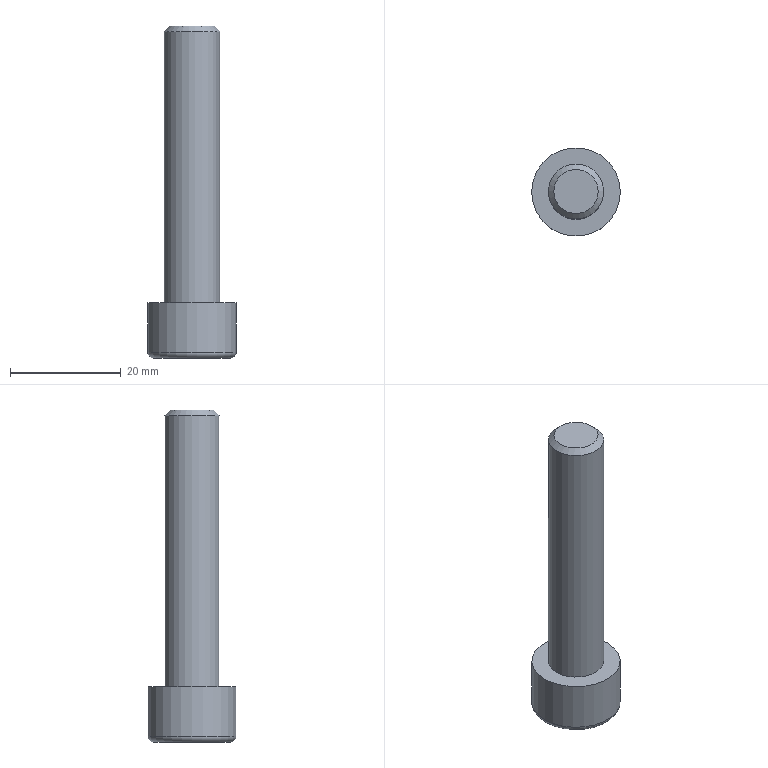Part | NX | features solid 2 | 1 solid | 14 faces | box 16 x 16 x 60 mm | volume 5614 mm3 | plane 9 | cylinder 2 | cone 2 | torus 1 | commonest cylinder face diameters 10 x1 16 x1
STEP:
#1=CARTESIAN_POINT('',(-600.5,-180.,-90.));
#2=VERTEX_POINT('',#1);
#3=CARTESIAN_POINT('',(-607.5,-180.,-90.));
#4=DIRECTION('',(0.,0.,1.));
#5=DIRECTION('',(1.,0.,0.));
#6=AXIS2_PLACEMENT_3D('',#3,#4,#5);
#7=CIRCLE('',#6,7.);
#8=EDGE_CURVE('',#2,#2,#7,.T.);
#9=ORIENTED_EDGE('',*,*,#8,.F.);
#10=EDGE_LOOP('',(#9));
#11=FACE_BOUND('',#10,.T.);
#12=CARTESIAN_POINT('',(-603.5,-182.309,-90.));
#13=VERTEX_POINT('',#12);
#14=CARTESIAN_POINT('',(-607.5,-184.619,-90.));
#15=VERTEX_POINT('',#14);
#16=CARTESIAN_POINT('',(-603.5,-182.309,-90.));
#17=DIRECTION('',(-0.866,-0.5,0.));
#18=VECTOR('',#17,1000.);
#19=LINE('',#16,#18);
#20=EDGE_CURVE('',#13,#15,#19,.T.);
#21=ORIENTED_EDGE('',*,*,#20,.F.);
#22=CARTESIAN_POINT('',(-603.5,-177.691,-90.));
#23=VERTEX_POINT('',#22);
#24=CARTESIAN_POINT('',(-603.5,-177.691,-90.));
#25=DIRECTION('',(0.,-1.,0.));
#26=VECTOR('',#25,1000.);
#27=LINE('',#24,#26);
#28=EDGE_CURVE('',#23,#13,#27,.T.);
#29=ORIENTED_EDGE('',*,*,#28,.F.);
#30=CARTESIAN_POINT('',(-607.5,-175.381,-90.));
#31=VERTEX_POINT('',#30);
#32=CARTESIAN_POINT('',(-607.5,-175.381,-90.));
#33=DIRECTION('',(0.866,-0.5,0.));
#34=VECTOR('',#33,1000.);
#35=LINE('',#32,#34);
#36=EDGE_CURVE('',#31,#23,#35,.T.);
#37=ORIENTED_EDGE('',*,*,#36,.F.);
#38=CARTESIAN_POINT('',(-611.5,-177.691,-90.));
#39=VERTEX_POINT('',#38);
#40=CARTESIAN_POINT('',(-611.5,-177.691,-90.));
#41=DIRECTION('',(0.866,0.5,0.));
#42=VECTOR('',#41,1000.);
#43=LINE('',#40,#42);
#44=EDGE_CURVE('',#39,#31,#43,.T.);
#45=ORIENTED_EDGE('',*,*,#44,.F.);
#46=CARTESIAN_POINT('',(-611.5,-182.309,-90.));
#47=VERTEX_POINT('',#46);
#48=CARTESIAN_POINT('',(-611.5,-182.309,-90.));
#49=DIRECTION('',(0.,1.,0.));
#50=VECTOR('',#49,1000.);
#51=LINE('',#48,#50);
#52=EDGE_CURVE('',#47,#39,#51,.T.);
#53=ORIENTED_EDGE('',*,*,#52,.F.);
#54=CARTESIAN_POINT('',(-607.5,-184.619,-90.));
#55=DIRECTION('',(-0.866,0.5,0.));
#56=VECTOR('',#55,1000.);
#57=LINE('',#54,#56);
#58=EDGE_CURVE('',#15,#47,#57,.T.);
#59=ORIENTED_EDGE('',*,*,#58,.F.);
#60=EDGE_LOOP('',(#21,#29,#37,#45,#53,#59));
#61=FACE_BOUND('',#60,.T.);
#62=CARTESIAN_POINT('',(-607.5,-180.,-90.));
#63=DIRECTION('',(0.,0.,-1.));
#64=DIRECTION('',(1.,0.,0.));
#65=AXIS2_PLACEMENT_3D('',#62,#63,#64);
#66=PLANE('',#65);
#67=ADVANCED_FACE('',(#11,#61),#66,.T.);
#68=CARTESIAN_POINT('',(-612.5,-180.,-80.));
#69=VERTEX_POINT('',#68);
#70=CARTESIAN_POINT('',(-607.5,-180.,-80.));
#71=DIRECTION('',(0.,0.,-1.));
#72=DIRECTION('',(-1.,0.,0.));
#73=AXIS2_PLACEMENT_3D('',#70,#71,#72);
#74=CIRCLE('',#73,5.);
#75=EDGE_CURVE('',#69,#69,#74,.T.);
#76=ORIENTED_EDGE('',*,*,#75,.T.);
#77=EDGE_LOOP('',(#76));
#78=FACE_BOUND('',#77,.T.);
#79=CARTESIAN_POINT('',(-599.5,-180.,-80.));
#80=VERTEX_POINT('',#79);
#81=CARTESIAN_POINT('',(-607.5,-180.,-80.));
#82=DIRECTION('',(0.,0.,1.));
#83=DIRECTION('',(1.,0.,0.));
#84=AXIS2_PLACEMENT_3D('',#81,#82,#83);
#85=CIRCLE('',#84,8.);
#86=EDGE_CURVE('',#80,#80,#85,.T.);
#87=ORIENTED_EDGE('',*,*,#86,.T.);
#88=EDGE_LOOP('',(#87));
#89=FACE_BOUND('',#88,.T.);
#90=CARTESIAN_POINT('',(-607.5,-180.,-80.));
#91=DIRECTION('',(0.,0.,1.));
#92=DIRECTION('',(-1.,0.,0.));
#93=AXIS2_PLACEMENT_3D('',#90,#91,#92);
#94=PLANE('',#93);
#95=ADVANCED_FACE('',(#78,#89),#94,.T.);
#96=CARTESIAN_POINT('',(-599.5,-180.,-89.));
#97=VERTEX_POINT('',#96);
#98=CARTESIAN_POINT('',(-607.5,-180.,-89.));
#99=DIRECTION('',(0.,0.,1.));
#100=DIRECTION('',(1.,0.,0.));
#101=AXIS2_PLACEMENT_3D('',#98,#99,#100);
#102=CIRCLE('',#101,8.);
#103=EDGE_CURVE('',#97,#97,#102,.F.);
#104=ORIENTED_EDGE('',*,*,#103,.F.);
#105=EDGE_LOOP('',(#104));
#106=FACE_BOUND('',#105,.T.);
#107=ORIENTED_EDGE('',*,*,#86,.F.);
#108=EDGE_LOOP('',(#107));
#109=FACE_BOUND('',#108,.T.);
#110=CARTESIAN_POINT('',(-607.5,-180.,-80.));
#111=DIRECTION('',(0.,0.,-1.));
#112=DIRECTION('',(1.,0.,0.));
#113=AXIS2_PLACEMENT_3D('',#110,#111,#112);
#114=CYLINDRICAL_SURFACE('',#113,8.);
#115=ADVANCED_FACE('',(#106,#109),#114,.T.);
#116=CARTESIAN_POINT('',(-607.5,-184.619,-85.667));
#117=VERTEX_POINT('',#116);
#118=CARTESIAN_POINT('',(-607.5,-184.619,-90.));
#119=DIRECTION('',(0.,0.,1.));
#120=VECTOR('',#119,1000.);
#121=LINE('',#118,#120);
#122=EDGE_CURVE('',#15,#117,#121,.T.);
#123=ORIENTED_EDGE('',*,*,#122,.T.);
#124=CARTESIAN_POINT('',(-603.5,-182.309,-85.667));
#125=VERTEX_POINT('',#124);
#126=CARTESIAN_POINT('',(-607.5,-184.619,-85.667));
#127=CARTESIAN_POINT('',(-606.847,-184.242,-85.449));
#128=CARTESIAN_POINT('',(-605.507,-183.468,-85.17));
#129=CARTESIAN_POINT('',(-604.154,-182.687,-85.449));
#130=CARTESIAN_POINT('',(-603.5,-182.309,-85.667));
#131=B_SPLINE_CURVE_WITH_KNOTS('',3,(#126,#127,#128,#129,#130),.UNSPECIFIED.,.F.,.F.,(4,1,4),(0.000000238,0.002333,0.004665),.UNSPECIFIED.);
#132=EDGE_CURVE('',#117,#125,#131,.T.);
#133=ORIENTED_EDGE('',*,*,#132,.T.);
#134=CARTESIAN_POINT('',(-603.5,-182.309,-90.));
#135=DIRECTION('',(0.,0.,1.));
#136=VECTOR('',#135,1000.);
#137=LINE('',#134,#136);
#138=EDGE_CURVE('',#13,#125,#137,.T.);
#139=ORIENTED_EDGE('',*,*,#138,.F.);
#140=ORIENTED_EDGE('',*,*,#20,.T.);
#141=EDGE_LOOP('',(#123,#133,#139,#140));
#142=FACE_BOUND('',#141,.T.);
#143=CARTESIAN_POINT('',(-605.5,-183.464,-86.5));
#144=DIRECTION('',(0.5,-0.866,0.));
#145=DIRECTION('',(0.866,0.5,0.));
#146=AXIS2_PLACEMENT_3D('',#143,#144,#145);
#147=PLANE('',#146);
#148=ADVANCED_FACE('',(#142),#147,.F.);
#149=ORIENTED_EDGE('',*,*,#138,.T.);
#150=CARTESIAN_POINT('',(-603.5,-177.691,-85.667));
#151=VERTEX_POINT('',#150);
#152=CARTESIAN_POINT('',(-603.5,-182.309,-85.667));
#153=CARTESIAN_POINT('',(-603.5,-181.558,-85.45));
#154=CARTESIAN_POINT('',(-603.5,-180.001,-85.168));
#155=CARTESIAN_POINT('',(-603.5,-178.437,-85.451));
#156=CARTESIAN_POINT('',(-603.5,-177.691,-85.667));
#157=B_SPLINE_CURVE_WITH_KNOTS('',3,(#152,#153,#154,#155,#156),.UNSPECIFIED.,.F.,.F.,(4,1,4),(0.004163,0.0065,0.008837),.UNSPECIFIED.);
#158=EDGE_CURVE('',#125,#151,#157,.T.);
#159=ORIENTED_EDGE('',*,*,#158,.T.);
#160=CARTESIAN_POINT('',(-603.5,-177.691,-90.));
#161=DIRECTION('',(0.,0.,1.));
#162=VECTOR('',#161,1000.);
#163=LINE('',#160,#162);
#164=EDGE_CURVE('',#23,#151,#163,.T.);
#165=ORIENTED_EDGE('',*,*,#164,.F.);
#166=ORIENTED_EDGE('',*,*,#28,.T.);
#167=EDGE_LOOP('',(#149,#159,#165,#166));
#168=FACE_BOUND('',#167,.T.);
#169=CARTESIAN_POINT('',(-603.5,-180.,-86.5));
#170=DIRECTION('',(1.,0.,0.));
#171=DIRECTION('',(0.,0.,1.));
#172=AXIS2_PLACEMENT_3D('',#169,#170,#171);
#173=PLANE('',#172);
#174=ADVANCED_FACE('',(#168),#173,.F.);
#175=ORIENTED_EDGE('',*,*,#164,.T.);
#176=CARTESIAN_POINT('',(-607.5,-175.381,-85.667));
#177=VERTEX_POINT('',#176);
#178=CARTESIAN_POINT('',(-603.5,-177.691,-85.667));
#179=CARTESIAN_POINT('',(-604.153,-177.314,-85.449));
#180=CARTESIAN_POINT('',(-605.493,-176.54,-85.17));
#181=CARTESIAN_POINT('',(-606.846,-175.759,-85.449));
#182=CARTESIAN_POINT('',(-607.5,-175.381,-85.667));
#183=B_SPLINE_CURVE_WITH_KNOTS('',3,(#178,#179,#180,#181,#182),.UNSPECIFIED.,.F.,.F.,(4,1,4),(0.000000238,0.002333,0.004665),.UNSPECIFIED.);
#184=EDGE_CURVE('',#151,#177,#183,.T.);
#185=ORIENTED_EDGE('',*,*,#184,.T.);
#186=CARTESIAN_POINT('',(-607.5,-175.381,-90.));
#187=DIRECTION('',(0.,0.,1.));
#188=VECTOR('',#187,1000.);
#189=LINE('',#186,#188);
#190=EDGE_CURVE('',#31,#177,#189,.T.);
#191=ORIENTED_EDGE('',*,*,#190,.F.);
#192=ORIENTED_EDGE('',*,*,#36,.T.);
#193=EDGE_LOOP('',(#175,#185,#191,#192));
#194=FACE_BOUND('',#193,.T.);
#195=CARTESIAN_POINT('',(-605.5,-176.536,-86.5));
#196=DIRECTION('',(0.5,0.866,0.));
#197=DIRECTION('',(-0.866,0.5,0.));
#198=AXIS2_PLACEMENT_3D('',#195,#196,#197);
#199=PLANE('',#198);
#200=ADVANCED_FACE('',(#194),#199,.F.);
#201=ORIENTED_EDGE('',*,*,#190,.T.);
#202=CARTESIAN_POINT('',(-611.5,-177.691,-85.667));
#203=VERTEX_POINT('',#202);
#204=CARTESIAN_POINT('',(-607.5,-175.381,-85.667));
#205=CARTESIAN_POINT('',(-608.153,-175.758,-85.449));
#206=CARTESIAN_POINT('',(-609.493,-176.532,-85.17));
#207=CARTESIAN_POINT('',(-610.846,-177.313,-85.449));
#208=CARTESIAN_POINT('',(-611.5,-177.691,-85.667));
#209=B_SPLINE_CURVE_WITH_KNOTS('',3,(#204,#205,#206,#207,#208),.UNSPECIFIED.,.F.,.F.,(4,1,4),(0.000000238,0.002333,0.004665),.UNSPECIFIED.);
#210=EDGE_CURVE('',#177,#203,#209,.T.);
#211=ORIENTED_EDGE('',*,*,#210,.T.);
#212=CARTESIAN_POINT('',(-611.5,-177.691,-90.));
#213=DIRECTION('',(0.,0.,1.));
#214=VECTOR('',#213,1000.);
#215=LINE('',#212,#214);
#216=EDGE_CURVE('',#39,#203,#215,.T.);
#217=ORIENTED_EDGE('',*,*,#216,.F.);
#218=ORIENTED_EDGE('',*,*,#44,.T.);
#219=EDGE_LOOP('',(#201,#211,#217,#218));
#220=FACE_BOUND('',#219,.T.);
#221=CARTESIAN_POINT('',(-609.5,-176.536,-86.5));
#222=DIRECTION('',(-0.5,0.866,0.));
#223=DIRECTION('',(-0.866,-0.5,0.));
#224=AXIS2_PLACEMENT_3D('',#221,#222,#223);
#225=PLANE('',#224);
#226=ADVANCED_FACE('',(#220),#225,.F.);
#227=ORIENTED_EDGE('',*,*,#216,.T.);
#228=CARTESIAN_POINT('',(-611.5,-182.309,-85.667));
#229=VERTEX_POINT('',#228);
#230=CARTESIAN_POINT('',(-611.5,-182.309,-85.667));
#231=CARTESIAN_POINT('',(-611.5,-181.558,-85.45));
#232=CARTESIAN_POINT('',(-611.5,-180.001,-85.168));
#233=CARTESIAN_POINT('',(-611.5,-178.437,-85.451));
#234=CARTESIAN_POINT('',(-611.5,-177.691,-85.667));
#235=B_SPLINE_CURVE_WITH_KNOTS('',3,(#230,#231,#232,#233,#234),.UNSPECIFIED.,.F.,.F.,(4,1,4),(0.004163,0.0065,0.008837),.UNSPECIFIED.);
#236=EDGE_CURVE('',#203,#229,#235,.F.);
#237=ORIENTED_EDGE('',*,*,#236,.T.);
#238=CARTESIAN_POINT('',(-611.5,-182.309,-90.));
#239=DIRECTION('',(0.,0.,1.));
#240=VECTOR('',#239,1000.);
#241=LINE('',#238,#240);
#242=EDGE_CURVE('',#47,#229,#241,.T.);
#243=ORIENTED_EDGE('',*,*,#242,.F.);
#244=ORIENTED_EDGE('',*,*,#52,.T.);
#245=EDGE_LOOP('',(#227,#237,#243,#244));
#246=FACE_BOUND('',#245,.T.);
#247=CARTESIAN_POINT('',(-611.5,-180.,-86.5));
#248=DIRECTION('',(-1.,0.,0.));
#249=DIRECTION('',(0.,0.,-1.));
#250=AXIS2_PLACEMENT_3D('',#247,#248,#249);
#251=PLANE('',#250);
#252=ADVANCED_FACE('',(#246),#251,.F.);
#253=ORIENTED_EDGE('',*,*,#242,.T.);
#254=CARTESIAN_POINT('',(-611.5,-182.309,-85.667));
#255=CARTESIAN_POINT('',(-610.847,-182.686,-85.449));
#256=CARTESIAN_POINT('',(-609.507,-183.46,-85.17));
#257=CARTESIAN_POINT('',(-608.154,-184.241,-85.449));
#258=CARTESIAN_POINT('',(-607.5,-184.619,-85.667));
#259=B_SPLINE_CURVE_WITH_KNOTS('',3,(#254,#255,#256,#257,#258),.UNSPECIFIED.,.F.,.F.,(4,1,4),(0.000000238,0.002333,0.004665),.UNSPECIFIED.);
#260=EDGE_CURVE('',#229,#117,#259,.T.);
#261=ORIENTED_EDGE('',*,*,#260,.T.);
#262=ORIENTED_EDGE('',*,*,#122,.F.);
#263=ORIENTED_EDGE('',*,*,#58,.T.);
#264=EDGE_LOOP('',(#253,#261,#262,#263));
#265=FACE_BOUND('',#264,.T.);
#266=CARTESIAN_POINT('',(-609.5,-183.464,-86.5));
#267=DIRECTION('',(-0.5,-0.866,0.));
#268=DIRECTION('',(0.866,-0.5,0.));
#269=AXIS2_PLACEMENT_3D('',#266,#267,#268);
#270=PLANE('',#269);
#271=ADVANCED_FACE('',(#265),#270,.F.);
#272=ORIENTED_EDGE('',*,*,#132,.F.);
#273=ORIENTED_EDGE('',*,*,#260,.F.);
#274=ORIENTED_EDGE('',*,*,#236,.F.);
#275=ORIENTED_EDGE('',*,*,#210,.F.);
#276=ORIENTED_EDGE('',*,*,#184,.F.);
#277=ORIENTED_EDGE('',*,*,#158,.F.);
#278=EDGE_LOOP('',(#272,#273,#274,#275,#276,#277));
#279=FACE_BOUND('',#278,.T.);
#280=CARTESIAN_POINT('',(-607.5,-180.,-83.));
#281=VERTEX_POINT('',#280);
#282=VERTEX_LOOP('',#281);
#283=FACE_BOUND('',#282,.T.);
#284=CARTESIAN_POINT('',(-607.5,-180.,-83.));
#285=DIRECTION('',(0.,0.,-1.));
#286=DIRECTION('',(1.,0.,0.));
#287=AXIS2_PLACEMENT_3D('',#284,#285,#286);
#288=CONICAL_SURFACE('',#287,0.,1.047);
#289=ADVANCED_FACE('',(#279,#283),#288,.F.);
#290=ORIENTED_EDGE('',*,*,#8,.T.);
#291=EDGE_LOOP('',(#290));
#292=FACE_BOUND('',#291,.T.);
#293=ORIENTED_EDGE('',*,*,#103,.T.);
#294=EDGE_LOOP('',(#293));
#295=FACE_BOUND('',#294,.T.);
#296=CARTESIAN_POINT('',(-607.5,-180.,-89.));
#297=DIRECTION('',(0.,0.,-1.));
#298=DIRECTION('',(1.,0.,0.));
#299=AXIS2_PLACEMENT_3D('',#296,#297,#298);
#300=TOROIDAL_SURFACE('',#299,7.,1.);
#301=ADVANCED_FACE('',(#292,#295),#300,.T.);
#302=CARTESIAN_POINT('',(-611.5,-180.,-30.));
#303=VERTEX_POINT('',#302);
#304=CARTESIAN_POINT('',(-607.5,-180.,-30.));
#305=DIRECTION('',(0.,0.,-1.));
#306=DIRECTION('',(-1.,0.,0.));
#307=AXIS2_PLACEMENT_3D('',#304,#305,#306);
#308=CIRCLE('',#307,4.);
#309=EDGE_CURVE('',#303,#303,#308,.T.);
#310=ORIENTED_EDGE('',*,*,#309,.F.);
#311=EDGE_LOOP('',(#310));
#312=FACE_BOUND('',#311,.T.);
#313=CARTESIAN_POINT('',(-607.5,-180.,-30.));
#314=DIRECTION('',(0.,0.,1.));
#315=DIRECTION('',(-1.,0.,0.));
#316=AXIS2_PLACEMENT_3D('',#313,#314,#315);
#317=PLANE('',#316);
#318=ADVANCED_FACE('',(#312),#317,.T.);
#319=CARTESIAN_POINT('',(-612.5,-180.,-31.));
#320=VERTEX_POINT('',#319);
#321=CARTESIAN_POINT('',(-607.5,-180.,-31.));
#322=DIRECTION('',(0.,0.,-1.));
#323=DIRECTION('',(-1.,0.,0.));
#324=AXIS2_PLACEMENT_3D('',#321,#322,#323);
#325=CIRCLE('',#324,5.);
#326=EDGE_CURVE('',#320,#320,#325,.F.);
#327=ORIENTED_EDGE('',*,*,#326,.F.);
#328=EDGE_LOOP('',(#327));
#329=FACE_BOUND('',#328,.T.);
#330=ORIENTED_EDGE('',*,*,#75,.F.);
#331=EDGE_LOOP('',(#330));
#332=FACE_BOUND('',#331,.T.);
#333=CARTESIAN_POINT('',(-607.5,-180.,-80.));
#334=DIRECTION('',(0.,0.,1.));
#335=DIRECTION('',(-1.,0.,0.));
#336=AXIS2_PLACEMENT_3D('',#333,#334,#335);
#337=CYLINDRICAL_SURFACE('',#336,5.);
#338=ADVANCED_FACE('',(#329,#332),#337,.T.);
#339=ORIENTED_EDGE('',*,*,#309,.T.);
#340=EDGE_LOOP('',(#339));
#341=FACE_BOUND('',#340,.T.);
#342=ORIENTED_EDGE('',*,*,#326,.T.);
#343=EDGE_LOOP('',(#342));
#344=FACE_BOUND('',#343,.T.);
#345=CARTESIAN_POINT('',(-607.5,-180.,-31.));
#346=DIRECTION('',(0.,0.,-1.));
#347=DIRECTION('',(1.,0.,0.));
#348=AXIS2_PLACEMENT_3D('',#345,#346,#347);
#349=CONICAL_SURFACE('',#348,5.,0.7854);
#350=ADVANCED_FACE('',(#341,#344),#349,.T.);
#351=CLOSED_SHELL('',(#67,#95,#115,#148,#174,#200,#226,#252,#271,#289,#301,#318,#338,#350));
#352=MANIFOLD_SOLID_BREP('',#351);
#353=(LENGTH_UNIT()NAMED_UNIT(*)SI_UNIT(.MILLI.,.METRE.));
#354=UNCERTAINTY_MEASURE_WITH_UNIT(LENGTH_MEASURE(0.0508),#353,'','');
#355=(NAMED_UNIT(*)PLANE_ANGLE_UNIT()SI_UNIT($,.RADIAN.));
#356=(NAMED_UNIT(*)SI_UNIT($,.STERADIAN.)SOLID_ANGLE_UNIT());
#357=(GEOMETRIC_REPRESENTATION_CONTEXT(3)GLOBAL_UNCERTAINTY_ASSIGNED_CONTEXT((#354))GLOBAL_UNIT_ASSIGNED_CONTEXT((#353,#355,#356))REPRESENTATION_CONTEXT('',''));
#358=ADVANCED_BREP_SHAPE_REPRESENTATION('',(#352),#357);